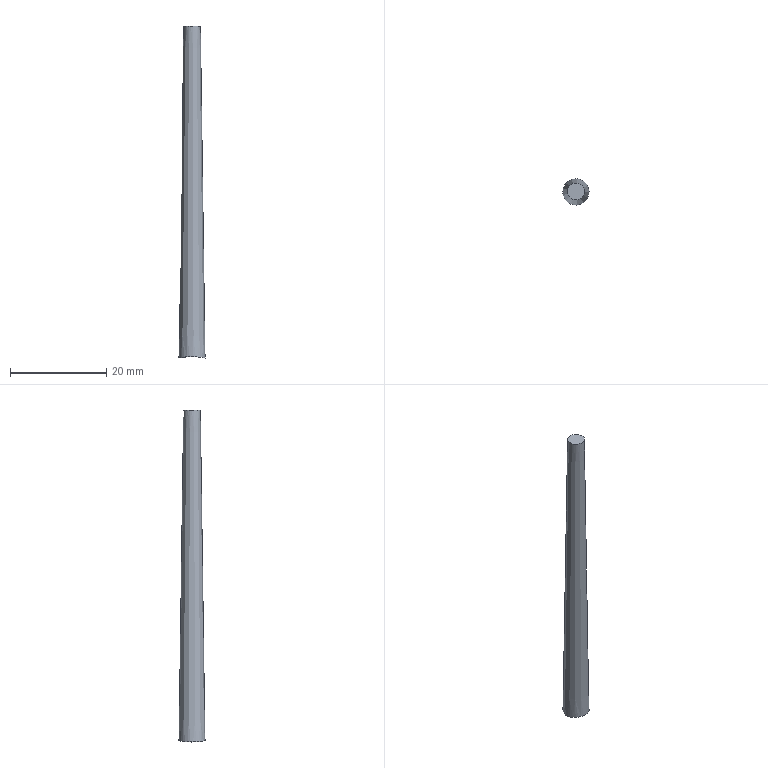Part | NX | features solid 2 | 1 solid | 3 faces | box 5.422 x 5.415 x 68.837 mm | volume 1088 mm3 | cone 1 | plane 1 | cylinder 1 | commonest cylinder face diameters 26.633 x1
STEP:
#1=CARTESIAN_POINT('',(-1.982,-1.847,21.893));
#2=VERTEX_POINT('',#1);
#3=CARTESIAN_POINT('',(-0.1016,-2.998,22.11));
#4=CARTESIAN_POINT('',(-2.197,-2.048,21.889));
#5=CARTESIAN_POINT('',(-3.003,0.1057,21.693));
#6=CARTESIAN_POINT('',(-2.05,2.193,21.918));
#7=CARTESIAN_POINT('',(0.104,2.998,22.11));
#8=CARTESIAN_POINT('',(2.195,2.048,21.889));
#9=CARTESIAN_POINT('',(3.003,-0.101,21.692));
#10=CARTESIAN_POINT('',(2.049,-2.194,21.918));
#11=CARTESIAN_POINT('',(-0.1016,-2.998,22.11));
#12=CARTESIAN_POINT('',(-2.197,-2.048,21.889));
#13=CARTESIAN_POINT('',(-3.003,0.1057,21.693));
#14=B_SPLINE_CURVE_WITH_KNOTS('',3,(#3,#4,#5,#6,#7,#8,#9,#10,#11,#12,#13),.UNSPECIFIED.,.T.,.F.,(1,1,1,1,1,1,1,1,1,1,1,1,1,1,1),(-0.006369,-0.004246,-0.002123,0.,0.002123,0.004246,0.006369,0.008492,0.01062,0.01274,0.01486,0.01698,0.01911,0.02123,0.02335),.UNSPECIFIED.);
#15=EDGE_CURVE('',#2,#2,#14,.T.);
#16=ORIENTED_EDGE('',*,*,#15,.F.);
#17=EDGE_LOOP('',(#16));
#18=FACE_BOUND('',#17,.T.);
#19=CARTESIAN_POINT('',(1.75,0.,90.6));
#20=VERTEX_POINT('',#19);
#21=CARTESIAN_POINT('',(0.,0.,90.6));
#22=DIRECTION('',(0.,0.,1.));
#23=DIRECTION('',(1.,0.,0.));
#24=AXIS2_PLACEMENT_3D('',#21,#22,#23);
#25=CIRCLE('',#24,1.75);
#26=EDGE_CURVE('',#20,#20,#25,.F.);
#27=ORIENTED_EDGE('',*,*,#26,.T.);
#28=EDGE_LOOP('',(#27));
#29=FACE_BOUND('',#28,.T.);
#30=CARTESIAN_POINT('',(0.,0.,90.6));
#31=DIRECTION('',(0.,0.,-1.));
#32=DIRECTION('',(1.,0.,0.));
#33=AXIS2_PLACEMENT_3D('',#30,#31,#32);
#34=CONICAL_SURFACE('',#33,1.75,0.01396);
#35=ADVANCED_FACE('',(#18,#29),#34,.T.);
#36=ORIENTED_EDGE('',*,*,#26,.F.);
#37=EDGE_LOOP('',(#36));
#38=FACE_BOUND('',#37,.T.);
#39=CARTESIAN_POINT('',(0.,0.,90.6));
#40=DIRECTION('',(0.,0.,1.));
#41=DIRECTION('',(1.,0.,0.));
#42=AXIS2_PLACEMENT_3D('',#39,#40,#41);
#43=PLANE('',#42);
#44=ADVANCED_FACE('',(#38),#43,.T.);
#45=ORIENTED_EDGE('',*,*,#15,.T.);
#46=EDGE_LOOP('',(#45));
#47=FACE_BOUND('',#46,.T.);
#48=CARTESIAN_POINT('',(0.,0.,8.725));
#49=DIRECTION('',(0.,-1.,0.));
#50=DIRECTION('',(1.,0.,0.));
#51=AXIS2_PLACEMENT_3D('',#48,#49,#50);
#52=CYLINDRICAL_SURFACE('',#51,13.316);
#53=ADVANCED_FACE('',(#47),#52,.F.);
#54=CLOSED_SHELL('',(#35,#44,#53));
#55=MANIFOLD_SOLID_BREP('',#54);
#56=(LENGTH_UNIT()NAMED_UNIT(*)SI_UNIT(.MILLI.,.METRE.));
#57=UNCERTAINTY_MEASURE_WITH_UNIT(LENGTH_MEASURE(0.0508),#56,'','');
#58=(NAMED_UNIT(*)PLANE_ANGLE_UNIT()SI_UNIT($,.RADIAN.));
#59=(NAMED_UNIT(*)SI_UNIT($,.STERADIAN.)SOLID_ANGLE_UNIT());
#60=(GEOMETRIC_REPRESENTATION_CONTEXT(3)GLOBAL_UNCERTAINTY_ASSIGNED_CONTEXT((#57))GLOBAL_UNIT_ASSIGNED_CONTEXT((#56,#58,#59))REPRESENTATION_CONTEXT('',''));
#61=ADVANCED_BREP_SHAPE_REPRESENTATION('',(#55),#60);